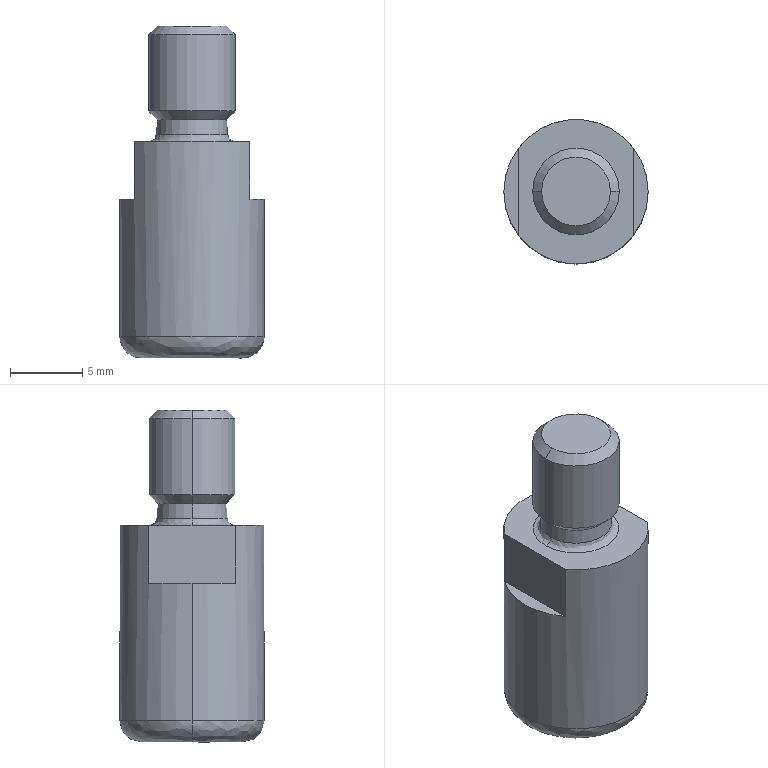Part | SolidWorks | features BaseBody 1 | 1 solid | 21 faces | box 10 x 10 x 23 mm | volume 1337 mm3 | plane 7 | cone 6 | cylinder 4 | spline 4 | commonest cylinder face diameters 6 x2 10 x2
STEP:
#1=CARTESIAN_POINT('',(-2.387,0.,8.));
#2=VERTEX_POINT('',#1);
#3=CARTESIAN_POINT('',(2.387,0.,8.));
#4=VERTEX_POINT('',#3);
#5=CARTESIAN_POINT('',(0.,0.,8.));
#6=DIRECTION('',(0.,0.,-1.));
#7=DIRECTION('',(-1.,0.,0.));
#8=AXIS2_PLACEMENT_3D('',#5,#6,#7);
#9=CIRCLE('',#8,2.387);
#10=EDGE_CURVE('',#2,#4,#9,.T.);
#11=ORIENTED_EDGE('',*,*,#10,.F.);
#12=CARTESIAN_POINT('',(0.,0.,8.));
#13=DIRECTION('',(0.,0.,-1.));
#14=DIRECTION('',(-1.,0.,0.));
#15=AXIS2_PLACEMENT_3D('',#12,#13,#14);
#16=CIRCLE('',#15,2.387);
#17=EDGE_CURVE('',#4,#2,#16,.T.);
#18=ORIENTED_EDGE('',*,*,#17,.F.);
#19=EDGE_LOOP('',(#11,#18));
#20=FACE_OUTER_BOUND('',#19,.T.);
#21=CARTESIAN_POINT('',(0.,0.,8.));
#22=DIRECTION('',(0.,0.,-1.));
#23=DIRECTION('',(0.,-1.,0.));
#24=AXIS2_PLACEMENT_3D('',#21,#22,#23);
#25=PLANE('',#24);
#26=ADVANCED_FACE('',(#20),#25,.F.);
#27=CARTESIAN_POINT('',(3.,0.,7.386));
#28=VERTEX_POINT('',#27);
#29=CARTESIAN_POINT('',(3.,0.,7.387));
#30=DIRECTION('',(0.7071,0.,-0.7071));
#31=VECTOR('',#30,1000.);
#32=LINE('',#29,#31);
#33=EDGE_CURVE('',#4,#28,#32,.T.);
#34=ORIENTED_EDGE('',*,*,#33,.F.);
#35=ORIENTED_EDGE('',*,*,#17,.T.);
#36=CARTESIAN_POINT('',(-3.,0.,7.386));
#37=VERTEX_POINT('',#36);
#38=CARTESIAN_POINT('',(-3.,0.,7.387));
#39=DIRECTION('',(-0.7071,0.,-0.7071));
#40=VECTOR('',#39,1000.);
#41=LINE('',#38,#40);
#42=EDGE_CURVE('',#2,#37,#41,.T.);
#43=ORIENTED_EDGE('',*,*,#42,.T.);
#44=CARTESIAN_POINT('',(0.,0.,7.386));
#45=DIRECTION('',(0.,0.,-1.));
#46=DIRECTION('',(1.,0.,0.));
#47=AXIS2_PLACEMENT_3D('',#44,#45,#46);
#48=CIRCLE('',#47,3.);
#49=EDGE_CURVE('',#28,#37,#48,.T.);
#50=ORIENTED_EDGE('',*,*,#49,.F.);
#51=EDGE_LOOP('',(#34,#35,#43,#50));
#52=FACE_OUTER_BOUND('',#51,.T.);
#53=CARTESIAN_POINT('',(0.,0.,7.387));
#54=DIRECTION('',(0.,0.,-1.));
#55=DIRECTION('',(-1.,0.,0.));
#56=AXIS2_PLACEMENT_3D('',#53,#54,#55);
#57=CONICAL_SURFACE('',#56,3.,0.7854);
#58=ADVANCED_FACE('',(#52),#57,.T.);
#59=CARTESIAN_POINT('',(-3.,0.,2.114));
#60=VERTEX_POINT('',#59);
#61=CARTESIAN_POINT('',(-3.,0.,-100.));
#62=DIRECTION('',(0.,0.,1.));
#63=VECTOR('',#62,1000.);
#64=LINE('',#61,#63);
#65=EDGE_CURVE('',#60,#37,#64,.T.);
#66=ORIENTED_EDGE('',*,*,#65,.F.);
#67=CARTESIAN_POINT('',(3.,0.,2.114));
#68=VERTEX_POINT('',#67);
#69=CARTESIAN_POINT('',(0.,0.,2.114));
#70=DIRECTION('',(0.,0.,-1.));
#71=DIRECTION('',(1.,0.,0.));
#72=AXIS2_PLACEMENT_3D('',#69,#70,#71);
#73=CIRCLE('',#72,3.);
#74=EDGE_CURVE('',#68,#60,#73,.T.);
#75=ORIENTED_EDGE('',*,*,#74,.F.);
#76=CARTESIAN_POINT('',(3.,0.,-100.));
#77=DIRECTION('',(0.,0.,1.));
#78=VECTOR('',#77,1000.);
#79=LINE('',#76,#78);
#80=EDGE_CURVE('',#68,#28,#79,.T.);
#81=ORIENTED_EDGE('',*,*,#80,.T.);
#82=ORIENTED_EDGE('',*,*,#49,.T.);
#83=EDGE_LOOP('',(#66,#75,#81,#82));
#84=FACE_OUTER_BOUND('',#83,.T.);
#85=CARTESIAN_POINT('',(0.,0.,-100.));
#86=DIRECTION('',(0.,0.,1.));
#87=DIRECTION('',(1.,0.,0.));
#88=AXIS2_PLACEMENT_3D('',#85,#86,#87);
#89=CYLINDRICAL_SURFACE('',#88,3.);
#90=ADVANCED_FACE('',(#84),#89,.T.);
#91=CARTESIAN_POINT('',(-2.387,0.,1.5));
#92=VERTEX_POINT('',#91);
#93=CARTESIAN_POINT('',(-3.,0.,2.114));
#94=DIRECTION('',(-0.7071,0.,0.7071));
#95=VECTOR('',#94,1000.);
#96=LINE('',#93,#95);
#97=EDGE_CURVE('',#92,#60,#96,.T.);
#98=ORIENTED_EDGE('',*,*,#97,.F.);
#99=CARTESIAN_POINT('',(2.387,0.,1.5));
#100=VERTEX_POINT('',#99);
#101=CARTESIAN_POINT('',(0.,0.,1.5));
#102=DIRECTION('',(0.,0.,-1.));
#103=DIRECTION('',(-1.,0.,0.));
#104=AXIS2_PLACEMENT_3D('',#101,#102,#103);
#105=CIRCLE('',#104,2.387);
#106=EDGE_CURVE('',#100,#92,#105,.T.);
#107=ORIENTED_EDGE('',*,*,#106,.F.);
#108=CARTESIAN_POINT('',(3.,0.,2.114));
#109=DIRECTION('',(0.7071,0.,0.7071));
#110=VECTOR('',#109,1000.);
#111=LINE('',#108,#110);
#112=EDGE_CURVE('',#100,#68,#111,.T.);
#113=ORIENTED_EDGE('',*,*,#112,.T.);
#114=ORIENTED_EDGE('',*,*,#74,.T.);
#115=EDGE_LOOP('',(#98,#107,#113,#114));
#116=FACE_OUTER_BOUND('',#115,.T.);
#117=CARTESIAN_POINT('',(0.,0.,2.114));
#118=DIRECTION('',(0.,0.,1.));
#119=DIRECTION('',(1.,0.,0.));
#120=AXIS2_PLACEMENT_3D('',#117,#118,#119);
#121=CONICAL_SURFACE('',#120,3.,0.7854);
#122=ADVANCED_FACE('',(#116),#121,.T.);
#123=CARTESIAN_POINT('',(2.465,0.,0.4623));
#124=VERTEX_POINT('',#123);
#125=CARTESIAN_POINT('',(2.465,0.,0.4623));
#126=DIRECTION('',(0.07545,0.,-0.9971));
#127=VECTOR('',#126,1000.);
#128=LINE('',#125,#127);
#129=EDGE_CURVE('',#100,#124,#128,.T.);
#130=ORIENTED_EDGE('',*,*,#129,.F.);
#131=ORIENTED_EDGE('',*,*,#106,.T.);
#132=CARTESIAN_POINT('',(-2.465,0.,0.4623));
#133=VERTEX_POINT('',#132);
#134=CARTESIAN_POINT('',(-2.465,0.,0.4623));
#135=DIRECTION('',(-0.07545,0.,-0.9971));
#136=VECTOR('',#135,1000.);
#137=LINE('',#134,#136);
#138=EDGE_CURVE('',#92,#133,#137,.T.);
#139=ORIENTED_EDGE('',*,*,#138,.T.);
#140=CARTESIAN_POINT('',(0.,0.,0.4623));
#141=DIRECTION('',(0.,0.,1.));
#142=DIRECTION('',(-1.,0.,0.));
#143=AXIS2_PLACEMENT_3D('',#140,#141,#142);
#144=CIRCLE('',#143,2.465);
#145=EDGE_CURVE('',#133,#124,#144,.T.);
#146=ORIENTED_EDGE('',*,*,#145,.T.);
#147=EDGE_LOOP('',(#130,#131,#139,#146));
#148=FACE_OUTER_BOUND('',#147,.T.);
#149=CARTESIAN_POINT('',(0.,0.,0.4623));
#150=DIRECTION('',(0.,0.,-1.));
#151=DIRECTION('',(-1.,0.,0.));
#152=AXIS2_PLACEMENT_3D('',#149,#150,#151);
#153=CONICAL_SURFACE('',#152,2.465,0.07552);
#154=ADVANCED_FACE('',(#148),#153,.T.);
#155=CARTESIAN_POINT('',(-3.5,0.,-15.));
#156=VERTEX_POINT('',#155);
#157=CARTESIAN_POINT('',(3.5,0.,-15.));
#158=VERTEX_POINT('',#157);
#159=CARTESIAN_POINT('',(-3.5,0.,-15.));
#160=CARTESIAN_POINT('',(-3.5,-7.,-15.));
#161=CARTESIAN_POINT('',(3.5,-7.,-15.));
#162=CARTESIAN_POINT('',(3.5,0.,-15.));
#163=(BOUNDED_CURVE()B_SPLINE_CURVE(3,(#159,#160,#161,#162),.UNSPECIFIED.,.F.,.F.)B_SPLINE_CURVE_WITH_KNOTS((4,4),(0.,0.5),.UNSPECIFIED.)CURVE()GEOMETRIC_REPRESENTATION_ITEM()RATIONAL_B_SPLINE_CURVE((1.,0.3333,0.3333,1.))REPRESENTATION_ITEM(''));
#164=EDGE_CURVE('',#156,#158,#163,.T.);
#165=ORIENTED_EDGE('',*,*,#164,.F.);
#166=CARTESIAN_POINT('',(3.5,0.,-15.));
#167=CARTESIAN_POINT('',(3.5,7.,-15.));
#168=CARTESIAN_POINT('',(-3.5,7.,-15.));
#169=CARTESIAN_POINT('',(-3.5,0.,-15.));
#170=(BOUNDED_CURVE()B_SPLINE_CURVE(3,(#166,#167,#168,#169),.UNSPECIFIED.,.F.,.F.)B_SPLINE_CURVE_WITH_KNOTS((4,4),(0.5,1.),.UNSPECIFIED.)CURVE()GEOMETRIC_REPRESENTATION_ITEM()RATIONAL_B_SPLINE_CURVE((1.,0.3333,0.3333,1.))REPRESENTATION_ITEM(''));
#171=EDGE_CURVE('',#158,#156,#170,.T.);
#172=ORIENTED_EDGE('',*,*,#171,.F.);
#173=EDGE_LOOP('',(#165,#172));
#174=FACE_OUTER_BOUND('',#173,.T.);
#175=CARTESIAN_POINT('',(0.,3.5,-15.));
#176=DIRECTION('',(0.,0.,1.));
#177=DIRECTION('',(1.,0.,0.));
#178=AXIS2_PLACEMENT_3D('',#175,#176,#177);
#179=PLANE('',#178);
#180=ADVANCED_FACE('',(#174),#179,.F.);
#181=CARTESIAN_POINT('',(2.964,0.,0.));
#182=VERTEX_POINT('',#181);
#183=CARTESIAN_POINT('',(2.964,0.,0.5));
#184=DIRECTION('',(0.,-1.,0.));
#185=DIRECTION('',(1.,0.,0.));
#186=AXIS2_PLACEMENT_3D('',#183,#184,#185);
#187=CIRCLE('',#186,0.5);
#188=EDGE_CURVE('',#124,#182,#187,.T.);
#189=ORIENTED_EDGE('',*,*,#188,.F.);
#190=ORIENTED_EDGE('',*,*,#145,.F.);
#191=CARTESIAN_POINT('',(-2.964,0.,0.));
#192=VERTEX_POINT('',#191);
#193=CARTESIAN_POINT('',(-2.964,0.,0.5));
#194=DIRECTION('',(0.,1.,0.));
#195=DIRECTION('',(-1.,0.,0.));
#196=AXIS2_PLACEMENT_3D('',#193,#194,#195);
#197=CIRCLE('',#196,0.5);
#198=EDGE_CURVE('',#133,#192,#197,.T.);
#199=ORIENTED_EDGE('',*,*,#198,.T.);
#200=CARTESIAN_POINT('',(-2.964,0.,0.));
#201=CARTESIAN_POINT('',(-2.964,-5.927,0.));
#202=CARTESIAN_POINT('',(2.964,-5.927,0.));
#203=CARTESIAN_POINT('',(2.964,0.,0.));
#204=(BOUNDED_CURVE()B_SPLINE_CURVE(3,(#200,#201,#202,#203),.UNSPECIFIED.,.F.,.F.)B_SPLINE_CURVE_WITH_KNOTS((4,4),(0.,0.5),.UNSPECIFIED.)CURVE()GEOMETRIC_REPRESENTATION_ITEM()RATIONAL_B_SPLINE_CURVE((1.,0.3333,0.3333,1.))REPRESENTATION_ITEM(''));
#205=EDGE_CURVE('',#192,#182,#204,.T.);
#206=ORIENTED_EDGE('',*,*,#205,.T.);
#207=EDGE_LOOP('',(#189,#190,#199,#206));
#208=FACE_OUTER_BOUND('',#207,.T.);
#209=CARTESIAN_POINT('',(2.465,0.,0.4623));
#210=CARTESIAN_POINT('',(2.465,-4.93,0.4623));
#211=CARTESIAN_POINT('',(-2.465,-4.93,0.4623));
#212=CARTESIAN_POINT('',(-2.465,0.,0.4623));
#213=CARTESIAN_POINT('',(2.486,0.,0.1874));
#214=CARTESIAN_POINT('',(2.486,-4.972,0.1874));
#215=CARTESIAN_POINT('',(-2.486,-4.972,0.1874));
#216=CARTESIAN_POINT('',(-2.486,0.,0.1874));
#217=CARTESIAN_POINT('',(2.688,0.,0.));
#218=CARTESIAN_POINT('',(2.688,-5.376,0.));
#219=CARTESIAN_POINT('',(-2.688,-5.376,0.));
#220=CARTESIAN_POINT('',(-2.688,0.,0.));
#221=CARTESIAN_POINT('',(2.964,0.,0.));
#222=CARTESIAN_POINT('',(2.964,-5.927,0.));
#223=CARTESIAN_POINT('',(-2.964,-5.927,0.));
#224=CARTESIAN_POINT('',(-2.964,0.,0.));
#225=(BOUNDED_SURFACE()B_SPLINE_SURFACE(3,3,((#209,#210,#211,#212),(#213,#214,#215,#216),(#217,#218,#219,#220),(#221,#222,#223,#224)),.UNSPECIFIED.,.F.,.F.,.F.)B_SPLINE_SURFACE_WITH_KNOTS((4,4),(4,4),(0.,1.),(0.,1.),.UNSPECIFIED.)GEOMETRIC_REPRESENTATION_ITEM()RATIONAL_B_SPLINE_SURFACE(((1.,0.3333,0.3333,1.),(0.8222,0.2741,0.2741,0.8222),(0.8222,0.2741,0.2741,0.8222),(1.,0.3333,0.3333,1.)))REPRESENTATION_ITEM('')SURFACE());
#226=ADVANCED_FACE('',(#208),#225,.F.);
#227=CARTESIAN_POINT('',(5.,0.,-13.5));
#228=VERTEX_POINT('',#227);
#229=CARTESIAN_POINT('',(3.5,0.,-13.5));
#230=DIRECTION('',(0.,-1.,0.));
#231=DIRECTION('',(1.,0.,0.));
#232=AXIS2_PLACEMENT_3D('',#229,#230,#231);
#233=CIRCLE('',#232,1.5);
#234=EDGE_CURVE('',#158,#228,#233,.T.);
#235=ORIENTED_EDGE('',*,*,#234,.F.);
#236=ORIENTED_EDGE('',*,*,#171,.T.);
#237=CARTESIAN_POINT('',(-5.,0.,-13.5));
#238=VERTEX_POINT('',#237);
#239=CARTESIAN_POINT('',(-3.5,0.,-13.5));
#240=DIRECTION('',(0.,1.,0.));
#241=DIRECTION('',(-1.,0.,0.));
#242=AXIS2_PLACEMENT_3D('',#239,#240,#241);
#243=CIRCLE('',#242,1.5);
#244=EDGE_CURVE('',#156,#238,#243,.T.);
#245=ORIENTED_EDGE('',*,*,#244,.T.);
#246=CARTESIAN_POINT('',(0.,0.,-13.5));
#247=DIRECTION('',(0.,0.,1.));
#248=DIRECTION('',(1.,0.,0.));
#249=AXIS2_PLACEMENT_3D('',#246,#247,#248);
#250=CIRCLE('',#249,5.);
#251=EDGE_CURVE('',#228,#238,#250,.T.);
#252=ORIENTED_EDGE('',*,*,#251,.F.);
#253=EDGE_LOOP('',(#235,#236,#245,#252));
#254=FACE_OUTER_BOUND('',#253,.T.);
#255=CARTESIAN_POINT('',(-3.5,0.,-15.));
#256=CARTESIAN_POINT('',(-3.5,7.,-15.));
#257=CARTESIAN_POINT('',(3.5,7.,-15.));
#258=CARTESIAN_POINT('',(3.5,0.,-15.));
#259=CARTESIAN_POINT('',(-4.379,0.,-15.));
#260=CARTESIAN_POINT('',(-4.379,8.757,-15.));
#261=CARTESIAN_POINT('',(4.379,8.757,-15.));
#262=CARTESIAN_POINT('',(4.379,0.,-15.));
#263=CARTESIAN_POINT('',(-5.,0.,-14.379));
#264=CARTESIAN_POINT('',(-5.,10.,-14.379));
#265=CARTESIAN_POINT('',(5.,10.,-14.379));
#266=CARTESIAN_POINT('',(5.,0.,-14.379));
#267=CARTESIAN_POINT('',(-5.,0.,-13.5));
#268=CARTESIAN_POINT('',(-5.,10.,-13.5));
#269=CARTESIAN_POINT('',(5.,10.,-13.5));
#270=CARTESIAN_POINT('',(5.,0.,-13.5));
#271=(BOUNDED_SURFACE()B_SPLINE_SURFACE(3,3,((#255,#256,#257,#258),(#259,#260,#261,#262),(#263,#264,#265,#266),(#267,#268,#269,#270)),.UNSPECIFIED.,.F.,.F.,.F.)B_SPLINE_SURFACE_WITH_KNOTS((4,4),(4,4),(0.,1.),(0.,1.),.UNSPECIFIED.)GEOMETRIC_REPRESENTATION_ITEM()RATIONAL_B_SPLINE_SURFACE(((1.,0.3333,0.3333,1.),(0.8047,0.2682,0.2682,0.8047),(0.8047,0.2682,0.2682,0.8047),(1.,0.3333,0.3333,1.)))REPRESENTATION_ITEM('')SURFACE());
#272=ADVANCED_FACE('',(#254),#271,.T.);
#273=CARTESIAN_POINT('',(-4.,-3.,-4.));
#274=VERTEX_POINT('',#273);
#275=CARTESIAN_POINT('',(-4.,3.,-4.));
#276=VERTEX_POINT('',#275);
#277=CARTESIAN_POINT('',(-4.,-3.,-4.));
#278=DIRECTION('',(0.,1.,0.));
#279=VECTOR('',#278,1000.);
#280=LINE('',#277,#279);
#281=EDGE_CURVE('',#274,#276,#280,.T.);
#282=ORIENTED_EDGE('',*,*,#281,.T.);
#283=CARTESIAN_POINT('',(-5.,0.,-4.));
#284=VERTEX_POINT('',#283);
#285=CARTESIAN_POINT('',(0.,0.,-4.));
#286=DIRECTION('',(0.,0.,-1.));
#287=DIRECTION('',(1.,0.,0.));
#288=AXIS2_PLACEMENT_3D('',#285,#286,#287);
#289=CIRCLE('',#288,5.);
#290=EDGE_CURVE('',#284,#276,#289,.T.);
#291=ORIENTED_EDGE('',*,*,#290,.F.);
#292=CARTESIAN_POINT('',(0.,0.,-4.));
#293=DIRECTION('',(0.,0.,-1.));
#294=DIRECTION('',(1.,0.,0.));
#295=AXIS2_PLACEMENT_3D('',#292,#293,#294);
#296=CIRCLE('',#295,5.);
#297=EDGE_CURVE('',#274,#284,#296,.T.);
#298=ORIENTED_EDGE('',*,*,#297,.F.);
#299=EDGE_LOOP('',(#282,#291,#298));
#300=FACE_OUTER_BOUND('',#299,.T.);
#301=CARTESIAN_POINT('',(0.,0.,-4.));
#302=DIRECTION('',(0.,0.,1.));
#303=DIRECTION('',(1.,0.,0.));
#304=AXIS2_PLACEMENT_3D('',#301,#302,#303);
#305=PLANE('',#304);
#306=ADVANCED_FACE('',(#300),#305,.T.);
#307=CARTESIAN_POINT('',(-4.,3.,0.));
#308=VERTEX_POINT('',#307);
#309=CARTESIAN_POINT('',(-4.,3.,-100.));
#310=DIRECTION('',(0.,0.,1.));
#311=VECTOR('',#310,1000.);
#312=LINE('',#309,#311);
#313=EDGE_CURVE('',#276,#308,#312,.T.);
#314=ORIENTED_EDGE('',*,*,#313,.F.);
#315=ORIENTED_EDGE('',*,*,#281,.F.);
#316=CARTESIAN_POINT('',(-4.,-3.,0.));
#317=VERTEX_POINT('',#316);
#318=CARTESIAN_POINT('',(-4.,-3.,-100.));
#319=DIRECTION('',(0.,0.,-1.));
#320=VECTOR('',#319,1000.);
#321=LINE('',#318,#320);
#322=EDGE_CURVE('',#317,#274,#321,.T.);
#323=ORIENTED_EDGE('',*,*,#322,.F.);
#324=CARTESIAN_POINT('',(-4.,2.964,0.));
#325=DIRECTION('',(0.,1.,0.));
#326=VECTOR('',#325,1000.);
#327=LINE('',#324,#326);
#328=EDGE_CURVE('',#317,#308,#327,.T.);
#329=ORIENTED_EDGE('',*,*,#328,.T.);
#330=EDGE_LOOP('',(#314,#315,#323,#329));
#331=FACE_OUTER_BOUND('',#330,.T.);
#332=CARTESIAN_POINT('',(-4.,-3.,-4.));
#333=DIRECTION('',(1.,0.,0.));
#334=DIRECTION('',(0.,1.,0.));
#335=AXIS2_PLACEMENT_3D('',#332,#333,#334);
#336=PLANE('',#335);
#337=ADVANCED_FACE('',(#331),#336,.F.);
#338=ORIENTED_EDGE('',*,*,#205,.F.);
#339=CARTESIAN_POINT('',(2.964,0.,0.));
#340=CARTESIAN_POINT('',(2.964,5.927,0.));
#341=CARTESIAN_POINT('',(-2.964,5.927,0.));
#342=CARTESIAN_POINT('',(-2.964,0.,0.));
#343=(BOUNDED_CURVE()B_SPLINE_CURVE(3,(#339,#340,#341,#342),.UNSPECIFIED.,.F.,.F.)B_SPLINE_CURVE_WITH_KNOTS((4,4),(0.5,1.),.UNSPECIFIED.)CURVE()GEOMETRIC_REPRESENTATION_ITEM()RATIONAL_B_SPLINE_CURVE((1.,0.3333,0.3333,1.))REPRESENTATION_ITEM(''));
#344=EDGE_CURVE('',#182,#192,#343,.T.);
#345=ORIENTED_EDGE('',*,*,#344,.F.);
#346=EDGE_LOOP('',(#338,#345));
#347=FACE_BOUND('',#346,.T.);
#348=ORIENTED_EDGE('',*,*,#328,.F.);
#349=CARTESIAN_POINT('',(4.,-3.,0.));
#350=VERTEX_POINT('',#349);
#351=CARTESIAN_POINT('',(0.,0.,0.));
#352=DIRECTION('',(0.,0.,-1.));
#353=DIRECTION('',(1.,0.,0.));
#354=AXIS2_PLACEMENT_3D('',#351,#352,#353);
#355=CIRCLE('',#354,5.);
#356=EDGE_CURVE('',#350,#317,#355,.T.);
#357=ORIENTED_EDGE('',*,*,#356,.F.);
#358=CARTESIAN_POINT('',(4.,3.,0.));
#359=VERTEX_POINT('',#358);
#360=CARTESIAN_POINT('',(4.,3.,0.));
#361=DIRECTION('',(0.,1.,0.));
#362=VECTOR('',#361,1000.);
#363=LINE('',#360,#362);
#364=EDGE_CURVE('',#350,#359,#363,.T.);
#365=ORIENTED_EDGE('',*,*,#364,.T.);
#366=CARTESIAN_POINT('',(0.,0.,0.));
#367=DIRECTION('',(0.,0.,-1.));
#368=DIRECTION('',(1.,0.,0.));
#369=AXIS2_PLACEMENT_3D('',#366,#367,#368);
#370=CIRCLE('',#369,5.);
#371=EDGE_CURVE('',#308,#359,#370,.T.);
#372=ORIENTED_EDGE('',*,*,#371,.F.);
#373=EDGE_LOOP('',(#348,#357,#365,#372));
#374=FACE_OUTER_BOUND('',#373,.T.);
#375=CARTESIAN_POINT('',(0.,2.964,0.));
#376=DIRECTION('',(0.,0.,-1.));
#377=DIRECTION('',(0.,-1.,0.));
#378=AXIS2_PLACEMENT_3D('',#375,#376,#377);
#379=PLANE('',#378);
#380=ADVANCED_FACE('',(#347,#374),#379,.F.);
#381=CARTESIAN_POINT('',(4.,3.,-4.));
#382=VERTEX_POINT('',#381);
#383=CARTESIAN_POINT('',(4.,-3.,-4.));
#384=VERTEX_POINT('',#383);
#385=CARTESIAN_POINT('',(4.,3.,-4.));
#386=DIRECTION('',(0.,-1.,0.));
#387=VECTOR('',#386,1000.);
#388=LINE('',#385,#387);
#389=EDGE_CURVE('',#382,#384,#388,.T.);
#390=ORIENTED_EDGE('',*,*,#389,.T.);
#391=CARTESIAN_POINT('',(5.,0.,-4.));
#392=VERTEX_POINT('',#391);
#393=CARTESIAN_POINT('',(0.,0.,-4.));
#394=DIRECTION('',(0.,0.,-1.));
#395=DIRECTION('',(1.,0.,0.));
#396=AXIS2_PLACEMENT_3D('',#393,#394,#395);
#397=CIRCLE('',#396,5.);
#398=EDGE_CURVE('',#392,#384,#397,.T.);
#399=ORIENTED_EDGE('',*,*,#398,.F.);
#400=CARTESIAN_POINT('',(0.,0.,-4.));
#401=DIRECTION('',(0.,0.,-1.));
#402=DIRECTION('',(1.,0.,0.));
#403=AXIS2_PLACEMENT_3D('',#400,#401,#402);
#404=CIRCLE('',#403,5.);
#405=EDGE_CURVE('',#382,#392,#404,.T.);
#406=ORIENTED_EDGE('',*,*,#405,.F.);
#407=EDGE_LOOP('',(#390,#399,#406));
#408=FACE_OUTER_BOUND('',#407,.T.);
#409=CARTESIAN_POINT('',(0.,0.,-4.));
#410=DIRECTION('',(0.,0.,1.));
#411=DIRECTION('',(1.,0.,0.));
#412=AXIS2_PLACEMENT_3D('',#409,#410,#411);
#413=PLANE('',#412);
#414=ADVANCED_FACE('',(#408),#413,.T.);
#415=CARTESIAN_POINT('',(4.,-3.,-100.));
#416=DIRECTION('',(0.,0.,1.));
#417=VECTOR('',#416,1000.);
#418=LINE('',#415,#417);
#419=EDGE_CURVE('',#384,#350,#418,.T.);
#420=ORIENTED_EDGE('',*,*,#419,.F.);
#421=ORIENTED_EDGE('',*,*,#389,.F.);
#422=CARTESIAN_POINT('',(4.,3.,-100.));
#423=DIRECTION('',(0.,0.,-1.));
#424=VECTOR('',#423,1000.);
#425=LINE('',#422,#424);
#426=EDGE_CURVE('',#359,#382,#425,.T.);
#427=ORIENTED_EDGE('',*,*,#426,.F.);
#428=ORIENTED_EDGE('',*,*,#364,.F.);
#429=EDGE_LOOP('',(#420,#421,#427,#428));
#430=FACE_OUTER_BOUND('',#429,.T.);
#431=CARTESIAN_POINT('',(4.,3.,-4.));
#432=DIRECTION('',(-1.,0.,0.));
#433=DIRECTION('',(0.,0.,1.));
#434=AXIS2_PLACEMENT_3D('',#431,#432,#433);
#435=PLANE('',#434);
#436=ADVANCED_FACE('',(#430),#435,.F.);
#437=CARTESIAN_POINT('',(-5.,0.,-100.));
#438=DIRECTION('',(0.,0.,1.));
#439=VECTOR('',#438,1000.);
#440=LINE('',#437,#439);
#441=EDGE_CURVE('',#238,#284,#440,.T.);
#442=ORIENTED_EDGE('',*,*,#441,.F.);
#443=CARTESIAN_POINT('',(0.,0.,-13.5));
#444=DIRECTION('',(0.,0.,1.));
#445=DIRECTION('',(1.,0.,0.));
#446=AXIS2_PLACEMENT_3D('',#443,#444,#445);
#447=CIRCLE('',#446,5.);
#448=EDGE_CURVE('',#238,#228,#447,.T.);
#449=ORIENTED_EDGE('',*,*,#448,.T.);
#450=CARTESIAN_POINT('',(5.,0.,-100.));
#451=DIRECTION('',(0.,0.,1.));
#452=VECTOR('',#451,1000.);
#453=LINE('',#450,#452);
#454=EDGE_CURVE('',#228,#392,#453,.T.);
#455=ORIENTED_EDGE('',*,*,#454,.T.);
#456=ORIENTED_EDGE('',*,*,#398,.T.);
#457=ORIENTED_EDGE('',*,*,#419,.T.);
#458=ORIENTED_EDGE('',*,*,#356,.T.);
#459=ORIENTED_EDGE('',*,*,#322,.T.);
#460=ORIENTED_EDGE('',*,*,#297,.T.);
#461=EDGE_LOOP('',(#442,#449,#455,#456,#457,#458,#459,#460));
#462=FACE_OUTER_BOUND('',#461,.T.);
#463=CARTESIAN_POINT('',(0.,0.,-100.));
#464=DIRECTION('',(0.,0.,1.));
#465=DIRECTION('',(1.,0.,0.));
#466=AXIS2_PLACEMENT_3D('',#463,#464,#465);
#467=CYLINDRICAL_SURFACE('',#466,5.);
#468=ADVANCED_FACE('',(#462),#467,.T.);
#469=ORIENTED_EDGE('',*,*,#10,.T.);
#470=ORIENTED_EDGE('',*,*,#33,.T.);
#471=CARTESIAN_POINT('',(0.,0.,7.386));
#472=DIRECTION('',(0.,0.,-1.));
#473=DIRECTION('',(1.,0.,0.));
#474=AXIS2_PLACEMENT_3D('',#471,#472,#473);
#475=CIRCLE('',#474,3.);
#476=EDGE_CURVE('',#37,#28,#475,.T.);
#477=ORIENTED_EDGE('',*,*,#476,.F.);
#478=ORIENTED_EDGE('',*,*,#42,.F.);
#479=EDGE_LOOP('',(#469,#470,#477,#478));
#480=FACE_OUTER_BOUND('',#479,.T.);
#481=CARTESIAN_POINT('',(0.,0.,7.387));
#482=DIRECTION('',(0.,0.,-1.));
#483=DIRECTION('',(-1.,0.,0.));
#484=AXIS2_PLACEMENT_3D('',#481,#482,#483);
#485=CONICAL_SURFACE('',#484,3.,0.7854);
#486=ADVANCED_FACE('',(#480),#485,.T.);
#487=CARTESIAN_POINT('',(0.,0.,2.114));
#488=DIRECTION('',(0.,0.,-1.));
#489=DIRECTION('',(1.,0.,0.));
#490=AXIS2_PLACEMENT_3D('',#487,#488,#489);
#491=CIRCLE('',#490,3.);
#492=EDGE_CURVE('',#60,#68,#491,.T.);
#493=ORIENTED_EDGE('',*,*,#492,.F.);
#494=ORIENTED_EDGE('',*,*,#65,.T.);
#495=ORIENTED_EDGE('',*,*,#476,.T.);
#496=ORIENTED_EDGE('',*,*,#80,.F.);
#497=EDGE_LOOP('',(#493,#494,#495,#496));
#498=FACE_OUTER_BOUND('',#497,.T.);
#499=CARTESIAN_POINT('',(0.,0.,-100.));
#500=DIRECTION('',(0.,0.,1.));
#501=DIRECTION('',(1.,0.,0.));
#502=AXIS2_PLACEMENT_3D('',#499,#500,#501);
#503=CYLINDRICAL_SURFACE('',#502,3.);
#504=ADVANCED_FACE('',(#498),#503,.T.);
#505=CARTESIAN_POINT('',(0.,0.,1.5));
#506=DIRECTION('',(0.,0.,-1.));
#507=DIRECTION('',(-1.,0.,0.));
#508=AXIS2_PLACEMENT_3D('',#505,#506,#507);
#509=CIRCLE('',#508,2.387);
#510=EDGE_CURVE('',#92,#100,#509,.T.);
#511=ORIENTED_EDGE('',*,*,#510,.F.);
#512=ORIENTED_EDGE('',*,*,#97,.T.);
#513=ORIENTED_EDGE('',*,*,#492,.T.);
#514=ORIENTED_EDGE('',*,*,#112,.F.);
#515=EDGE_LOOP('',(#511,#512,#513,#514));
#516=FACE_OUTER_BOUND('',#515,.T.);
#517=CARTESIAN_POINT('',(0.,0.,2.114));
#518=DIRECTION('',(0.,0.,1.));
#519=DIRECTION('',(1.,0.,0.));
#520=AXIS2_PLACEMENT_3D('',#517,#518,#519);
#521=CONICAL_SURFACE('',#520,3.,0.7854);
#522=ADVANCED_FACE('',(#516),#521,.T.);
#523=ORIENTED_EDGE('',*,*,#510,.T.);
#524=ORIENTED_EDGE('',*,*,#129,.T.);
#525=CARTESIAN_POINT('',(0.,0.,0.4623));
#526=DIRECTION('',(0.,0.,1.));
#527=DIRECTION('',(-1.,0.,0.));
#528=AXIS2_PLACEMENT_3D('',#525,#526,#527);
#529=CIRCLE('',#528,2.465);
#530=EDGE_CURVE('',#124,#133,#529,.T.);
#531=ORIENTED_EDGE('',*,*,#530,.T.);
#532=ORIENTED_EDGE('',*,*,#138,.F.);
#533=EDGE_LOOP('',(#523,#524,#531,#532));
#534=FACE_OUTER_BOUND('',#533,.T.);
#535=CARTESIAN_POINT('',(0.,0.,0.4623));
#536=DIRECTION('',(0.,0.,-1.));
#537=DIRECTION('',(-1.,0.,0.));
#538=AXIS2_PLACEMENT_3D('',#535,#536,#537);
#539=CONICAL_SURFACE('',#538,2.465,0.07552);
#540=ADVANCED_FACE('',(#534),#539,.T.);
#541=ORIENTED_EDGE('',*,*,#251,.T.);
#542=ORIENTED_EDGE('',*,*,#441,.T.);
#543=ORIENTED_EDGE('',*,*,#290,.T.);
#544=ORIENTED_EDGE('',*,*,#313,.T.);
#545=ORIENTED_EDGE('',*,*,#371,.T.);
#546=ORIENTED_EDGE('',*,*,#426,.T.);
#547=ORIENTED_EDGE('',*,*,#405,.T.);
#548=ORIENTED_EDGE('',*,*,#454,.F.);
#549=EDGE_LOOP('',(#541,#542,#543,#544,#545,#546,#547,#548));
#550=FACE_OUTER_BOUND('',#549,.T.);
#551=CARTESIAN_POINT('',(0.,0.,-100.));
#552=DIRECTION('',(0.,0.,1.));
#553=DIRECTION('',(1.,0.,0.));
#554=AXIS2_PLACEMENT_3D('',#551,#552,#553);
#555=CYLINDRICAL_SURFACE('',#554,5.);
#556=ADVANCED_FACE('',(#550),#555,.T.);
#557=ORIENTED_EDGE('',*,*,#530,.F.);
#558=ORIENTED_EDGE('',*,*,#188,.T.);
#559=ORIENTED_EDGE('',*,*,#344,.T.);
#560=ORIENTED_EDGE('',*,*,#198,.F.);
#561=EDGE_LOOP('',(#557,#558,#559,#560));
#562=FACE_OUTER_BOUND('',#561,.T.);
#563=CARTESIAN_POINT('',(-2.465,0.,0.4623));
#564=CARTESIAN_POINT('',(-2.465,4.93,0.4623));
#565=CARTESIAN_POINT('',(2.465,4.93,0.4623));
#566=CARTESIAN_POINT('',(2.465,0.,0.4623));
#567=CARTESIAN_POINT('',(-2.486,0.,0.1874));
#568=CARTESIAN_POINT('',(-2.486,4.972,0.1874));
#569=CARTESIAN_POINT('',(2.486,4.972,0.1874));
#570=CARTESIAN_POINT('',(2.486,0.,0.1874));
#571=CARTESIAN_POINT('',(-2.688,0.,0.));
#572=CARTESIAN_POINT('',(-2.688,5.376,0.));
#573=CARTESIAN_POINT('',(2.688,5.376,0.));
#574=CARTESIAN_POINT('',(2.688,0.,0.));
#575=CARTESIAN_POINT('',(-2.964,0.,0.));
#576=CARTESIAN_POINT('',(-2.964,5.927,0.));
#577=CARTESIAN_POINT('',(2.964,5.927,0.));
#578=CARTESIAN_POINT('',(2.964,0.,0.));
#579=(BOUNDED_SURFACE()B_SPLINE_SURFACE(3,3,((#563,#564,#565,#566),(#567,#568,#569,#570),(#571,#572,#573,#574),(#575,#576,#577,#578)),.UNSPECIFIED.,.F.,.F.,.F.)B_SPLINE_SURFACE_WITH_KNOTS((4,4),(4,4),(0.,1.),(0.,1.),.UNSPECIFIED.)GEOMETRIC_REPRESENTATION_ITEM()RATIONAL_B_SPLINE_SURFACE(((1.,0.3333,0.3333,1.),(0.8222,0.2741,0.2741,0.8222),(0.8222,0.2741,0.2741,0.8222),(1.,0.3333,0.3333,1.)))REPRESENTATION_ITEM('')SURFACE());
#580=ADVANCED_FACE('',(#562),#579,.F.);
#581=ORIENTED_EDGE('',*,*,#164,.T.);
#582=ORIENTED_EDGE('',*,*,#234,.T.);
#583=ORIENTED_EDGE('',*,*,#448,.F.);
#584=ORIENTED_EDGE('',*,*,#244,.F.);
#585=EDGE_LOOP('',(#581,#582,#583,#584));
#586=FACE_OUTER_BOUND('',#585,.T.);
#587=CARTESIAN_POINT('',(3.5,0.,-15.));
#588=CARTESIAN_POINT('',(3.5,-7.,-15.));
#589=CARTESIAN_POINT('',(-3.5,-7.,-15.));
#590=CARTESIAN_POINT('',(-3.5,0.,-15.));
#591=CARTESIAN_POINT('',(4.379,0.,-15.));
#592=CARTESIAN_POINT('',(4.379,-8.757,-15.));
#593=CARTESIAN_POINT('',(-4.379,-8.757,-15.));
#594=CARTESIAN_POINT('',(-4.379,0.,-15.));
#595=CARTESIAN_POINT('',(5.,0.,-14.379));
#596=CARTESIAN_POINT('',(5.,-10.,-14.379));
#597=CARTESIAN_POINT('',(-5.,-10.,-14.379));
#598=CARTESIAN_POINT('',(-5.,0.,-14.379));
#599=CARTESIAN_POINT('',(5.,0.,-13.5));
#600=CARTESIAN_POINT('',(5.,-10.,-13.5));
#601=CARTESIAN_POINT('',(-5.,-10.,-13.5));
#602=CARTESIAN_POINT('',(-5.,0.,-13.5));
#603=(BOUNDED_SURFACE()B_SPLINE_SURFACE(3,3,((#587,#588,#589,#590),(#591,#592,#593,#594),(#595,#596,#597,#598),(#599,#600,#601,#602)),.UNSPECIFIED.,.F.,.F.,.F.)B_SPLINE_SURFACE_WITH_KNOTS((4,4),(4,4),(0.,1.),(0.,1.),.UNSPECIFIED.)GEOMETRIC_REPRESENTATION_ITEM()RATIONAL_B_SPLINE_SURFACE(((1.,0.3333,0.3333,1.),(0.8047,0.2682,0.2682,0.8047),(0.8047,0.2682,0.2682,0.8047),(1.,0.3333,0.3333,1.)))REPRESENTATION_ITEM('')SURFACE());
#604=ADVANCED_FACE('',(#586),#603,.T.);
#605=CLOSED_SHELL('',(#26,#58,#90,#122,#154,#180,#226,#272,#306,#337,#380,#414,#436,#468,#486,#504,#522,#540,#556,#580,#604));
#606=MANIFOLD_SOLID_BREP('',#605);
#607=CARTESIAN_POINT('',(0.,0.,0.));
#608=DIRECTION('',(0.,0.,1.));
#609=DIRECTION('',(1.,0.,0.));
#610=AXIS2_PLACEMENT_3D('',#607,#608,#609);
#611=(LENGTH_UNIT()NAMED_UNIT(*)SI_UNIT(.MILLI.,.METRE.));
#612=UNCERTAINTY_MEASURE_WITH_UNIT(LENGTH_MEASURE(0.00001),#611,'','');
#613=(NAMED_UNIT(*)PLANE_ANGLE_UNIT()SI_UNIT($,.RADIAN.));
#614=(NAMED_UNIT(*)SI_UNIT($,.STERADIAN.)SOLID_ANGLE_UNIT());
#615=(GEOMETRIC_REPRESENTATION_CONTEXT(3)GLOBAL_UNCERTAINTY_ASSIGNED_CONTEXT((#612))GLOBAL_UNIT_ASSIGNED_CONTEXT((#611,#613,#614))REPRESENTATION_CONTEXT('',''));
#616=ADVANCED_BREP_SHAPE_REPRESENTATION('',(#606,#610),#615);